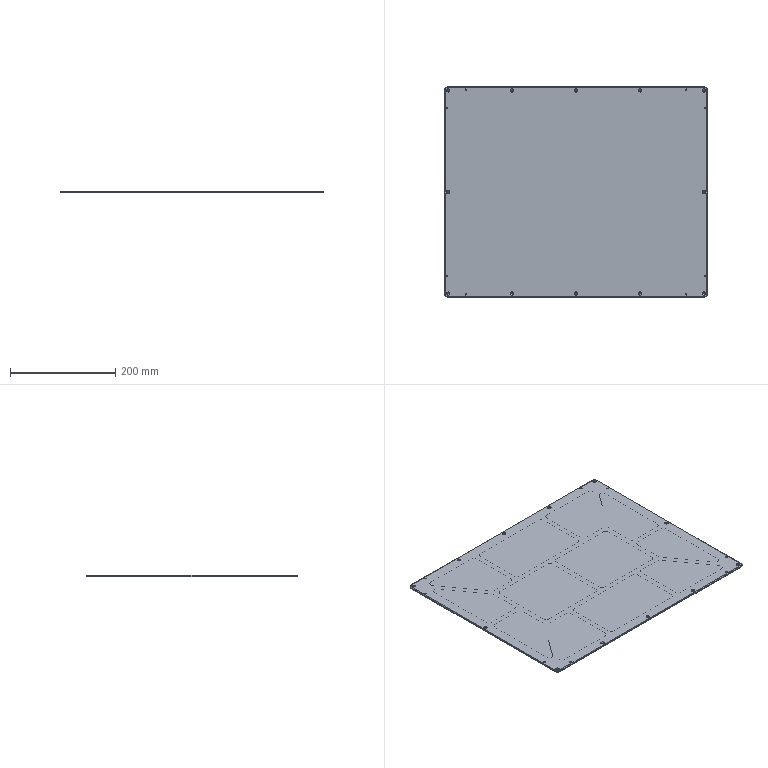NC program | Mastercam | posted with a generic post | part box 500 x 400 x 3 mm
Lines 2042 to 3034 of 11256:
(8 FEM |TOOL - 8|DIA. OFF. - 8|LEN. - 8|TOOL DIA. - 8.)
N4158 T8 M6
N4160 G0 G54 G90 X-136.27 Y140.355 C0. B0. S7000 M3
N4162 G43 H8 Z50.
N4164 Z1.
N4166 G1 Z.333 F600.
N4168 X-138.465 Z.314 F3500.
N4170 X-140.67 Z.295
N4172 X-145.964 Z.257
N4174 X-143.536 Y137.017
N4176 X-140.948 Y133.459 Z.219
N4178 X-138.36 Y129.9 Z.181
N4180 X-134.645 Y124.791 Z.144
N4182 Y127.543
N4184 Y131.943 Z.106
N4186 Y136.343 Z.068
N4188 Y140.355 Z.033
N4190 X-136.452 Z.03
N4192 X-138.465 Z.012
N4194 X-140.852 Z-.008
N4196 X-145.964 Z-.046
N4198 X-145.081 Y139.141
N4200 X-142.493 Y135.583 Z-.084
N4202 X-139.906 Y132.025 Z-.122
N4204 X-137.318 Y128.466 Z-.16
N4206 X-134.645 Y124.791 Z-.198
N4208 Y124.971
N4210 Y129.371 Z-.236
N4212 Y133.771 Z-.274
N4214 Y138.171 Z-.312
N4216 Y140.355 Z-.331
N4218 X-138.465 Z-.35
N4220 G3 X-139.29 Y139.53 J-.825
N4222 X-139.262 Y139.318 I.825
N4224 G1 X-138.595 Y136.809
N4226 G3 X-138.465 Y136.536 I.798 J.212
N4228 G2 X-139.246 Y137.097 J.825
N4230 G1 X-140.158 Y139.794
N4232 G3 X-140.94 Y140.355 I-.782 J-.264
N4234 G1 X-145.964
N4236 X-134.645 Y124.791
N4238 Y140.355
N4240 X-140.94
N4242 G2 X-141.729 Y140.941 J.825
N4244 G1 X-142.625 Y143.904
N4246 G3 X-143.415 Y144.49 I-.79 J-.239
N4248 G1 X-154.084
N4250 X-130.51 Y112.075
N4252 Y144.49
N4254 X-143.415
N4256 G2 X-144.207 Y145.085 J.825
N4258 G1 X-145.097 Y148.154
N4260 G3 X-145.89 Y148.749 I-.793 J-.23
N4262 G1 X-162.447
N4264 X-131.54 Y106.251
N4266 X-126.251
N4268 Y148.749
N4270 X-145.89
N4272 G2 X-146.687 Y149.361 J.825
N4274 G1 X-147.567 Y152.662
N4276 G3 X-148.365 Y153.274 I-.798 J-.213
N4278 G1 X-171.334
N4280 X-133.844 Y101.726
N4282 X-121.726
N4284 Y153.274
N4286 X-148.365
N4288 G2 X-149.162 Y153.886 J.825
N4290 G1 X-150.042 Y157.187
N4292 G3 X-150.84 Y157.799 I-.798 J-.213
N4294 G1 X-180.22
N4296 X-136.149 Y97.201
N4298 X-117.201
N4300 Y157.799
N4302 X-150.84
N4304 G2 X-151.637 Y158.411 J.825
N4306 G1 X-152.517 Y161.712
N4308 G3 X-153.315 Y162.324 I-.798 J-.213
N4310 G1 X-189.106
N4312 X-138.453 Y92.676
N4314 X-112.676
N4316 Y162.324
N4318 X-153.315
N4320 G2 X-154.112 Y162.937 J.825
N4322 G1 X-154.992 Y166.237
N4324 G3 X-155.79 Y166.85 I-.798 J-.212
N4326 G1 X-197.993
N4328 X-140.757 Y88.15
N4330 X-108.15
N4332 Y166.85
N4334 X-155.79
N4336 G2 X-156.587 Y167.462 J.825
N4338 G1 X-157.467 Y170.762
N4340 G3 X-158.265 Y171.375 I-.798 J-.212
N4342 G1 X-206.88
N4344 X-143.062 Y83.625
N4346 X-103.625
N4348 Y171.375
N4350 X-158.265
N4352 G2 X-159.062 Y171.987 J.825
N4354 G1 X-159.942 Y175.288
N4356 G3 X-160.74 Y175.9 I-.798 J-.213
N4358 G1 X-210.496
N4360 X-211.127 Y175.879
N4362 X-211.757 Y175.773
N4364 G3 X-212.449 Y175.426 I1.634 J-4.119
N4366 X-213.433 Y173.534 I1.398 J-1.929
N4368 G1 X-213.357 Y172.903
N4370 X-213.245 Y172.579
N4372 G3 X-212.669 Y171.642 I9.36 J5.107
N4374 G1 X-146.185 Y80.226
N4376 X-145.554 Y79.574
N4378 G3 X-144.613 Y79.165 I1.565 J2.311
N4380 G1 X-143.663 Y79.1
N4382 X-102.05
N4384 X-101.419 Y79.122
N4386 X-100.789 Y79.231
N4388 G3 X-100.108 Y79.574 I-1.685 J4.186
N4390 X-99.34 Y80.51 I-1.549 J2.054
N4392 G1 X-99.219 Y80.835
N4394 X-99.118 Y81.466
N4396 X-99.1 Y172.903
N4398 X-99.118 Y173.534
N4400 X-99.219 Y174.165
N4402 G3 X-99.791 Y175.151 I-2.451 J-.764
N4404 X-100.789 Y175.769 I-1.843 J-1.86
N4406 G1 X-101.419 Y175.878
N4408 X-102.05 Y175.9
N4410 X-160.74
N4412 G0 Z50.
N4414 X-136.27 Y140.355
N4416 Z.65
N4418 G1 Z-.017 F600.
N4420 X-138.465 Z-.036 F3500.
N4422 X-140.67 Z-.055
N4424 X-145.964 Z-.093
N4426 X-143.536 Y137.017
N4428 X-140.948 Y133.459 Z-.131
N4430 X-138.36 Y129.9 Z-.169
N4432 X-134.645 Y124.791 Z-.206
N4434 Y127.543
N4436 Y131.943 Z-.244
N4438 Y136.343 Z-.282
N4440 Y140.355 Z-.317
N4442 X-136.452 Z-.32
N4444 X-138.465 Z-.338
N4446 X-140.852 Z-.358
N4448 X-145.964 Z-.396
N4450 X-145.081 Y139.141
N4452 X-142.493 Y135.583 Z-.434
N4454 X-139.906 Y132.025 Z-.472
N4456 X-137.318 Y128.466 Z-.51
N4458 X-134.645 Y124.791 Z-.548
N4460 Y124.971
N4462 Y129.371 Z-.586
N4464 Y133.771 Z-.624
N4466 Y138.171 Z-.662
N4468 Y140.355 Z-.681
N4470 X-138.465 Z-.7
N4472 G3 X-139.29 Y139.53 J-.825
N4474 X-139.262 Y139.318 I.825
N4476 G1 X-138.595 Y136.809
N4478 G3 X-138.465 Y136.536 I.798 J.212
N4480 G2 X-139.246 Y137.097 J.825
N4482 G1 X-140.158 Y139.794
N4484 G3 X-140.94 Y140.355 I-.782 J-.264
N4486 G1 X-145.964
N4488 X-134.645 Y124.791
N4490 Y140.355
N4492 X-140.94
N4494 G2 X-141.729 Y140.941 J.825
N4496 G1 X-142.625 Y143.904
N4498 G3 X-143.415 Y144.49 I-.79 J-.239
N4500 G1 X-154.084
N4502 X-130.51 Y112.075
N4504 Y144.49
N4506 X-143.415
N4508 G2 X-144.207 Y145.085 J.825
N4510 G1 X-145.097 Y148.154
N4512 G3 X-145.89 Y148.749 I-.793 J-.23
N4514 G1 X-162.447
N4516 X-131.54 Y106.251
N4518 X-126.251
N4520 Y148.749
N4522 X-145.89
N4524 G2 X-146.687 Y149.361 J.825
N4526 G1 X-147.567 Y152.662
N4528 G3 X-148.365 Y153.274 I-.798 J-.213
N4530 G1 X-171.334
N4532 X-133.844 Y101.726
N4534 X-121.726
N4536 Y153.274
N4538 X-148.365
N4540 G2 X-149.162 Y153.886 J.825
N4542 G1 X-150.042 Y157.187
N4544 G3 X-150.84 Y157.799 I-.798 J-.213
N4546 G1 X-180.22
N4548 X-136.149 Y97.201
N4550 X-117.201
N4552 Y157.799
N4554 X-150.84
N4556 G2 X-151.637 Y158.411 J.825
N4558 G1 X-152.517 Y161.712
N4560 G3 X-153.315 Y162.324 I-.798 J-.213
N4562 G1 X-189.106
N4564 X-138.453 Y92.676
N4566 X-112.676
N4568 Y162.324
N4570 X-153.315
N4572 G2 X-154.112 Y162.937 J.825
N4574 G1 X-154.992 Y166.237
N4576 G3 X-155.79 Y166.85 I-.798 J-.212
N4578 G1 X-197.993
N4580 X-140.757 Y88.15
N4582 X-108.15
N4584 Y166.85
N4586 X-155.79
N4588 G2 X-156.587 Y167.462 J.825
N4590 G1 X-157.467 Y170.762
N4592 G3 X-158.265 Y171.375 I-.798 J-.212
N4594 G1 X-206.88
N4596 X-143.062 Y83.625
N4598 X-103.625
N4600 Y171.375
N4602 X-158.265
N4604 G2 X-159.062 Y171.987 J.825
N4606 G1 X-159.942 Y175.288
N4608 G3 X-160.74 Y175.9 I-.798 J-.213
N4610 G1 X-210.496
N4612 X-211.127 Y175.879
N4614 X-211.757 Y175.773
N4616 G3 X-212.449 Y175.426 I1.634 J-4.119
N4618 X-213.433 Y173.534 I1.398 J-1.929
N4620 G1 X-213.357 Y172.903
N4622 X-213.245 Y172.579
N4624 G3 X-212.669 Y171.642 I9.36 J5.107
N4626 G1 X-146.185 Y80.226
N4628 X-145.554 Y79.574
N4630 G3 X-144.613 Y79.165 I1.565 J2.311
N4632 G1 X-143.663 Y79.1
N4634 X-102.05
N4636 X-101.419 Y79.122
N4638 X-100.789 Y79.231
N4640 G3 X-100.108 Y79.574 I-1.685 J4.186
N4642 X-99.34 Y80.51 I-1.549 J2.054
N4644 G1 X-99.219 Y80.835
N4646 X-99.118 Y81.466
N4648 X-99.1 Y172.903
N4650 X-99.118 Y173.534
N4652 X-99.219 Y174.165
N4654 G3 X-99.791 Y175.151 I-2.451 J-.764
N4656 X-100.789 Y175.769 I-1.843 J-1.86
N4658 G1 X-101.419 Y175.878
N4660 X-102.05 Y175.9
N4662 X-160.74
N4664 G0 Z50.
N4666 X-136.27 Y140.355
N4668 Z.3
N4670 G1 Z-.367 F600.
N4672 X-138.465 Z-.386 F3500.
N4674 X-140.67 Z-.405
N4676 X-145.964 Z-.443
N4678 X-143.536 Y137.017
N4680 X-140.948 Y133.459 Z-.481
N4682 X-138.36 Y129.9 Z-.519
N4684 X-134.645 Y124.791 Z-.556
N4686 Y127.543
N4688 Y131.943 Z-.594
N4690 Y136.343 Z-.632
N4692 Y140.355 Z-.667
N4694 X-136.452 Z-.67
N4696 X-138.465 Z-.688
N4698 X-140.852 Z-.708
N4700 X-145.964 Z-.746
N4702 X-145.081 Y139.141
N4704 X-142.493 Y135.583 Z-.784
N4706 X-139.906 Y132.025 Z-.822
N4708 X-137.318 Y128.466 Z-.86
N4710 X-134.645 Y124.791 Z-.898
N4712 Y124.971
N4714 Y129.371 Z-.936
N4716 Y133.771 Z-.974
N4718 Y138.171 Z-1.012
N4720 Y140.355 Z-1.031
N4722 X-138.465 Z-1.05
N4724 G3 X-139.29 Y139.53 J-.825
N4726 X-139.262 Y139.318 I.825
N4728 G1 X-138.595 Y136.809
N4730 G3 X-138.465 Y136.536 I.798 J.212
N4732 G2 X-139.246 Y137.097 J.825
N4734 G1 X-140.158 Y139.794
N4736 G3 X-140.94 Y140.355 I-.782 J-.264
N4738 G1 X-145.964
N4740 X-134.645 Y124.791
N4742 Y140.355
N4744 X-140.94
N4746 G2 X-141.729 Y140.941 J.825
N4748 G1 X-142.625 Y143.904
N4750 G3 X-143.415 Y144.49 I-.79 J-.239
N4752 G1 X-154.084
N4754 X-130.51 Y112.075
N4756 Y144.49
N4758 X-143.415
N4760 G2 X-144.207 Y145.085 J.825
N4762 G1 X-145.097 Y148.154
N4764 G3 X-145.89 Y148.749 I-.793 J-.23
N4766 G1 X-162.447
N4768 X-131.54 Y106.251
N4770 X-126.251
N4772 Y148.749
N4774 X-145.89
N4776 G2 X-146.687 Y149.361 J.825
N4778 G1 X-147.567 Y152.662
N4780 G3 X-148.365 Y153.274 I-.798 J-.213
N4782 G1 X-171.334
N4784 X-133.844 Y101.726
N4786 X-121.726
N4788 Y153.274
N4790 X-148.365
N4792 G2 X-149.162 Y153.886 J.825
N4794 G1 X-150.042 Y157.187
N4796 G3 X-150.84 Y157.799 I-.798 J-.213
N4798 G1 X-180.22
N4800 X-136.149 Y97.201
N4802 X-117.201
N4804 Y157.799
N4806 X-150.84
N4808 G2 X-151.637 Y158.411 J.825
N4810 G1 X-152.517 Y161.712
N4812 G3 X-153.315 Y162.324 I-.798 J-.213
N4814 G1 X-189.106
N4816 X-138.453 Y92.676
N4818 X-112.676
N4820 Y162.324
N4822 X-153.315
N4824 G2 X-154.112 Y162.937 J.825
N4826 G1 X-154.992 Y166.237
N4828 G3 X-155.79 Y166.85 I-.798 J-.212
N4830 G1 X-197.993
N4832 X-140.757 Y88.15
N4834 X-108.15
N4836 Y166.85
N4838 X-155.79
N4840 G2 X-156.587 Y167.462 J.825
N4842 G1 X-157.467 Y170.762
N4844 G3 X-158.265 Y171.375 I-.798 J-.212
N4846 G1 X-206.88
N4848 X-143.062 Y83.625
N4850 X-103.625
N4852 Y171.375
N4854 X-158.265
N4856 G2 X-159.062 Y171.987 J.825
N4858 G1 X-159.942 Y175.288
N4860 G3 X-160.74 Y175.9 I-.798 J-.213
N4862 G1 X-210.496
N4864 X-211.127 Y175.879
N4866 X-211.757 Y175.773
N4868 G3 X-212.449 Y175.426 I1.634 J-4.119
N4870 X-213.433 Y173.534 I1.398 J-1.929
N4872 G1 X-213.357 Y172.903
N4874 X-213.245 Y172.579
N4876 G3 X-212.669 Y171.642 I9.36 J5.107
N4878 G1 X-146.185 Y80.226
N4880 X-145.554 Y79.574
N4882 G3 X-144.613 Y79.165 I1.565 J2.311
N4884 G1 X-143.663 Y79.1
N4886 X-102.05
N4888 X-101.419 Y79.122
N4890 X-100.789 Y79.231
N4892 G3 X-100.108 Y79.574 I-1.685 J4.186
N4894 X-99.34 Y80.51 I-1.549 J2.054
N4896 G1 X-99.219 Y80.835
N4898 X-99.118 Y81.466
N4900 X-99.1 Y172.903
N4902 X-99.118 Y173.534
N4904 X-99.219 Y174.165
N4906 G3 X-99.791 Y175.151 I-2.451 J-.764
N4908 X-100.789 Y175.769 I-1.843 J-1.86
N4910 G1 X-101.419 Y175.878
N4912 X-102.05 Y175.9
N4914 X-160.74
N4916 G0 Z50.
N4918 X-136.27 Y140.355
N4920 Z-.05
N4922 G1 Z-.717 F600.
N4924 X-138.465 Z-.736 F3500.
N4926 X-140.67 Z-.755
N4928 X-145.964 Z-.793
N4930 X-143.536 Y137.017
N4932 X-140.948 Y133.459 Z-.831
N4934 X-138.36 Y129.9 Z-.869
N4936 X-134.645 Y124.791 Z-.906
N4938 Y127.543
N4940 Y131.943 Z-.944
N4942 Y136.343 Z-.982
N4944 Y140.355 Z-1.017
N4946 X-136.452 Z-1.02
N4948 X-138.465 Z-1.038
N4950 X-140.852 Z-1.058
N4952 X-145.964 Z-1.096
N4954 X-145.081 Y139.141
N4956 X-142.493 Y135.583 Z-1.134
N4958 X-139.906 Y132.025 Z-1.172
N4960 X-137.318 Y128.466 Z-1.21
N4962 X-134.645 Y124.791 Z-1.248
N4964 Y124.971
N4966 Y129.371 Z-1.286
N4968 Y133.771 Z-1.324
N4970 Y138.171 Z-1.362
N4972 Y140.355 Z-1.381
N4974 X-138.465 Z-1.4
N4976 G3 X-139.29 Y139.53 J-.825
N4978 X-139.262 Y139.318 I.825
N4980 G1 X-138.595 Y136.809
N4982 G3 X-138.465 Y136.536 I.798 J.212
N4984 G2 X-139.246 Y137.097 J.825
N4986 G1 X-140.158 Y139.794
N4988 G3 X-140.94 Y140.355 I-.782 J-.264
N4990 G1 X-145.964
N4992 X-134.645 Y124.791
N4994 Y140.355
N4996 X-140.94
N4998 G2 X-141.729 Y140.941 J.825
N5000 G1 X-142.625 Y143.904
N5002 G3 X-143.415 Y144.49 I-.79 J-.239
N5004 G1 X-154.084
N5006 X-130.51 Y112.075
N5008 Y144.49
N5010 X-143.415
N5012 G2 X-144.207 Y145.085 J.825
N5014 G1 X-145.097 Y148.154
N5016 G3 X-145.89 Y148.749 I-.793 J-.23
N5018 G1 X-162.447
N5020 X-131.54 Y106.251
N5022 X-126.251
N5024 Y148.749
N5026 X-145.89
N5028 G2 X-146.687 Y149.361 J.825
N5030 G1 X-147.567 Y152.662
N5032 G3 X-148.365 Y153.274 I-.798 J-.213
N5034 G1 X-171.334
N5036 X-133.844 Y101.726
N5038 X-121.726
N5040 Y153.274
N5042 X-148.365
N5044 G2 X-149.162 Y153.886 J.825
N5046 G1 X-150.042 Y157.187
N5048 G3 X-150.84 Y157.799 I-.798 J-.213
N5050 G1 X-180.22
N5052 X-136.149 Y97.201
N5054 X-117.201
N5056 Y157.799
N5058 X-150.84
N5060 G2 X-151.637 Y158.411 J.825
N5062 G1 X-152.517 Y161.712
N5064 G3 X-153.315 Y162.324 I-.798 J-.213
N5066 G1 X-189.106
N5068 X-138.453 Y92.676
N5070 X-112.676
N5072 Y162.324
N5074 X-153.315
N5076 G2 X-154.112 Y162.937 J.825
N5078 G1 X-154.992 Y166.237
N5080 G3 X-155.79 Y166.85 I-.798 J-.212
N5082 G1 X-197.993
N5084 X-140.757 Y88.15
N5086 X-108.15
N5088 Y166.85
N5090 X-155.79
N5092 G2 X-156.587 Y167.462 J.825
N5094 G1 X-157.467 Y170.762
N5096 G3 X-158.265 Y171.375 I-.798 J-.212
N5098 G1 X-206.88
N5100 X-143.062 Y83.625
N5102 X-103.625
N5104 Y171.375
N5106 X-158.265
N5108 G2 X-159.062 Y171.987 J.825
N5110 G1 X-159.942 Y175.288
N5112 G3 X-160.74 Y175.9 I-.798 J-.213
N5114 G1 X-210.496
N5116 X-211.127 Y175.879
N5118 X-211.757 Y175.773
N5120 G3 X-212.449 Y175.426 I1.634 J-4.119
N5122 X-213.433 Y173.534 I1.398 J-1.929
N5124 G1 X-213.357 Y172.903
N5126 X-213.245 Y172.579
N5128 G3 X-212.669 Y171.642 I9.36 J5.107
N5130 G1 X-146.185 Y80.226
N5132 X-145.554 Y79.574
N5134 G3 X-144.613 Y79.165 I1.565 J2.311
N5136 G1 X-143.663 Y79.1
N5138 X-102.05
N5140 X-101.419 Y79.122
N5142 X-100.789 Y79.231
N5144 G3 X-100.108 Y79.574 I-1.685 J4.186
N5146 X-99.34 Y80.51 I-1.549 J2.054
N5148 G1 X-99.219 Y80.835
N5150 X-99.118 Y81.466
N5152 X-99.1 Y172.903
N5154 X-99.118 Y173.534
N5156 X-99.219 Y174.165
N5158 G3 X-99.791 Y175.151 I-2.451 J-.764
N5160 X-100.789 Y175.769 I-1.843 J-1.86
N5162 G1 X-101.419 Y175.878
N5164 X-102.05 Y175.9
N5166 X-160.74
N5168 G0 Z50.
N5170 X-136.27 Y140.355
N5172 Z-.4
N5174 G1 Z-.817 F600.
N5176 X-138.465 Z-.836 F1000.
N5178 X-140.67 Z-.855
N5180 X-145.964 Z-.893
N5182 X-143.536 Y137.017
N5184 X-140.948 Y133.459 Z-.931
N5186 X-138.36 Y129.9 Z-.969
N5188 X-134.645 Y124.791 Z-1.006
N5190 Y127.543
N5192 Y131.943 Z-1.044
N5194 Y136.343 Z-1.082
N5196 Y140.355 Z-1.117
N5198 X-136.452 Z-1.12
N5200 X-138.465 Z-1.138
N5202 X-140.852 Z-1.158
N5204 X-145.964 Z-1.196
N5206 X-145.081 Y139.141
N5208 X-142.493 Y135.583 Z-1.234
N5210 X-139.906 Y132.025 Z-1.272
N5212 X-137.318 Y128.466 Z-1.31
N5214 X-134.645 Y124.791 Z-1.348
N5216 Y124.971
N5218 Y129.371 Z-1.386
N5220 Y133.771 Z-1.424
N5222 Y138.171 Z-1.462
N5224 Y140.355 Z-1.481
N5226 X-138.465 Z-1.5
N5228 G3 X-139.29 Y139.53 J-.825 F3500.
N5230 X-139.262 Y139.318 I.825
N5232 G1 X-138.595 Y136.809
N5234 G3 X-138.465 Y136.536 I.798 J.212
N5236 G2 X-139.246 Y137.097 J.825
N5238 G1 X-140.158 Y139.794
N5240 G3 X-140.94 Y140.355 I-.782 J-.264
N5242 G1 X-145.964 F1000.
N5244 X-134.645 Y124.791
N5246 Y140.355
N5248 X-140.94
N5250 G2 X-141.729 Y140.941 J.825 F3500.
N5252 G1 X-142.625 Y143.904
N5254 G3 X-143.415 Y144.49 I-.79 J-.239
N5256 G1 X-154.084 F1000.
N5258 X-130.51 Y112.075
N5260 Y144.49
N5262 X-143.415
N5264 G2 X-144.207 Y145.085 J.825 F3500.
N5266 G1 X-145.097 Y148.154
N5268 G3 X-145.89 Y148.749 I-.793 J-.23
N5270 G1 X-162.447 F1000.
N5272 X-131.54 Y106.251
N5274 X-126.251
N5276 Y148.749
N5278 X-145.89
N5280 G2 X-146.687 Y149.361 J.825 F3500.
N5282 G1 X-147.567 Y152.662
N5284 G3 X-148.365 Y153.274 I-.798 J-.213
N5286 G1 X-171.334 F1000.
N5288 X-133.844 Y101.726
N5290 X-121.726
N5292 Y153.274
N5294 X-148.365
N5296 G2 X-149.162 Y153.886 J.825 F3500.
N5298 G1 X-150.042 Y157.187
N5300 G3 X-150.84 Y157.799 I-.798 J-.213
N5302 G1 X-180.22 F1000.
N5304 X-136.149 Y97.201
N5306 X-117.201
N5308 Y157.799
N5310 X-150.84
N5312 G2 X-151.637 Y158.411 J.825 F3500.
N5314 G1 X-152.517 Y161.712
N5316 G3 X-153.315 Y162.324 I-.798 J-.213
N5318 G1 X-189.106 F1000.
N5320 X-138.453 Y92.676
N5322 X-112.676
N5324 Y162.324
N5326 X-153.315
N5328 G2 X-154.112 Y162.937 J.825 F3500.
N5330 G1 X-154.992 Y166.237
N5332 G3 X-155.79 Y166.85 I-.798 J-.212
N5334 G1 X-197.993 F1000.
N5336 X-140.757 Y88.15
N5338 X-108.15
N5340 Y166.85
N5342 X-155.79
N5344 G2 X-156.587 Y167.462 J.825 F3500.
N5346 G1 X-157.467 Y170.762
N5348 G3 X-158.265 Y171.375 I-.798 J-.212
N5350 G1 X-206.88 F1000.
N5352 X-143.062 Y83.625
N5354 X-103.625
N5356 Y171.375
N5358 X-158.265
N5360 G2 X-159.062 Y171.987 J.825 F3500.
N5362 G1 X-159.942 Y175.288
N5364 G3 X-160.74 Y175.9 I-.798 J-.213
N5366 G1 X-210.496 F1000.
N5368 X-211.127 Y175.879
N5370 X-211.757 Y175.773
N5372 G3 X-212.449 Y175.426 I1.634 J-4.119
N5374 X-213.433 Y173.534 I1.398 J-1.929
N5376 G1 X-213.357 Y172.903
N5378 X-213.245 Y172.579
N5380 G3 X-212.669 Y171.642 I9.36 J5.107
N5382 G1 X-146.185 Y80.226
N5384 X-145.554 Y79.574
N5386 G3 X-144.613 Y79.165 I1.565 J2.311
N5388 G1 X-143.663 Y79.1
N5390 X-102.05
N5392 X-101.419 Y79.122
N5394 X-100.789 Y79.231
N5396 G3 X-100.108 Y79.574 I-1.685 J4.186
N5398 X-99.34 Y80.51 I-1.549 J2.054
N5400 G1 X-99.219 Y80.835
N5402 X-99.118 Y81.466
N5404 X-99.1 Y172.903
N5406 X-99.118 Y173.534
N5408 X-99.219 Y174.165
N5410 G3 X-99.791 Y175.151 I-2.451 J-.764
N5412 X-100.789 Y175.769 I-1.843 J-1.86
N5414 G1 X-101.419 Y175.878
N5416 X-102.05 Y175.9
N5418 X-160.74
N5420 G0 Z50.
N5422 X-10.062 Y125.983
N5424 Z1.
N5426 G1 Z.333 F600.
N5428 X-5.662 Z.295 F3500.
N5430 X-1.262 Z.257
N5432 X3.138 Z.219
N5434 X7.538 Z.181
N5436 X11.938 Z.144
N5438 X16.338 Z.106
N5440 X20.738 Z.068
N5442 X25.138 Z.03
N5444 X29.538 Z-.008
N5446 X34.017 Z-.046
N5448 Y129.017
N5450 X32.725
N5452 X28.325 Z-.084
N5454 X23.925 Z-.122
N5456 X19.525 Z-.16
N5458 X15.125 Z-.198
N5460 X10.725 Z-.236
N5462 X6.325 Z-.274
N5464 X1.925 Z-.312
N5466 X0. Z-.329
N5468 X-2.475 Z-.35
N5470 X-34.017
N5472 Y125.983
N5474 X34.017
N5476 Y129.017
N5478 X0.
N5480 X-2.475
N5482 G2 X-3.281 Y129.664 J.825
N5484 G1 X-4.144 Y133.579
N5486 G3 X-4.95 Y134.226 I-.806 J-.178
N5488 G1 X-39.226
N5490 Y120.774
N5492 X39.226
N5494 Y134.226
N5496 X0.
N5498 X-4.95
N5500 G2 X-5.756 Y134.873 J.825
N5502 G1 X-6.619 Y138.788
N5504 G3 X-7.425 Y139.435 I-.806 J-.178
N5506 G1 X-44.435
N5508 Y115.565
N5510 X44.435
N5512 Y139.435
N5514 X0.
N5516 X-7.425
N5518 G2 X-8.231 Y140.083 J.825
N5520 G1 X-9.094 Y143.998
N5522 G3 X-9.9 Y144.645 I-.806 J-.178
N5524 G1 X-49.645
N5526 Y110.355
N5528 X49.645
N5530 Y144.645
N5532 X0.
N5534 X-9.9
N5536 G2 X-10.706 Y145.292 J.825
N5538 G1 X-11.569 Y149.207
N5540 G3 X-12.375 Y149.854 I-.806 J-.178
N5542 G1 X-54.854
N5544 Y105.146
N5546 X54.854
N5548 Y149.854
N5550 X0.
N5552 X-12.375
N5554 G2 X-13.181 Y150.501 J.825
N5556 G1 X-14.044 Y154.416
N5558 G3 X-14.85 Y155.063 I-.806 J-.178
N5560 G1 X-60.063
N5562 Y99.937
N5564 X60.063
N5566 Y155.063
N5568 X0.
N5570 X-14.85
N5572 G2 X-15.656 Y155.711 J.825
N5574 G1 X-16.519 Y159.625
N5576 G3 X-17.325 Y160.273 I-.806 J-.177
N5578 G1 X-65.273
N5580 Y94.727
N5582 X65.273
N5584 Y160.273
N5586 X0.
N5588 X-17.325
N5590 G2 X-18.131 Y160.92 J.825
N5592 G1 X-18.994 Y164.834
N5594 G3 X-19.8 Y165.482 I-.806 J-.177
N5596 G1 X-70.482
N5598 Y89.518
N5600 X70.482
N5602 Y165.482
N5604 X0.
N5606 X-19.8
N5608 G2 X-20.606 Y166.129 J.825
N5610 G1 X-21.469 Y170.044
N5612 G3 X-22.275 Y170.691 I-.806 J-.178
N5614 G1 X-75.691
N5616 Y84.309
N5618 X75.691
N5620 Y170.691
N5622 X0.
N5624 X-22.275
N5626 G2 X-23.081 Y171.338 J.825
N5628 G1 X-23.944 Y175.253
N5630 G3 X-24.75 Y175.9 I-.806 J-.178
N5632 G1 X-78.199
N5634 X-78.83 Y175.856
N5636 X-79.314 Y175.741
N5638 G3 X-80.091 Y175.269 I1.466 J-3.285
N5640 X-80.722 Y174.357 I1.955 J-2.027
N5642 X-80.9 Y173.221 I3.526 J-1.136
N5644 G1 Y173.219
N5646 Y81.781
N5648 Y81.779
N5650 G3 X-80.722 Y80.643 I3.704
N5652 X-80.091 Y79.731 I2.586 J1.115
N5654 X-79.314 Y79.259 I2.243 J2.813
N5656 G1 X-78.83 Y79.144
N5658 X-78.199 Y79.1
N5660 X78.199
N5662 X78.83 Y79.144
N5664 X79.314 Y79.259
N5666 G3 X80.091 Y79.731 I-1.466 J3.285
N5668 X80.722 Y80.643 I-1.955 J2.027
N5670 X80.9 Y81.779 I-3.526 J1.136
N5672 G1 Y81.781
N5674 Y173.219
N5676 Y173.221
N5678 G3 X80.722 Y174.357 I-3.704
N5680 X80.091 Y175.269 I-2.586 J-1.115
N5682 X79.314 Y175.741 I-2.243 J-2.813
N5684 G1 X78.83 Y175.856
N5686 X78.199 Y175.9
N5688 X0.
N5690 X-24.75
N5692 G0 Z50.
N5694 X-10.062 Y125.983
N5696 Z.65
N5698 G1 Z-.017 F600.
N5700 X-5.662 Z-.055 F3500.
N5702 X-1.262 Z-.093
N5704 X3.138 Z-.131
N5706 X7.538 Z-.169
N5708 X11.938 Z-.206
N5710 X16.338 Z-.244
N5712 X20.738 Z-.282
N5714 X25.138 Z-.32
N5716 X29.538 Z-.358
N5718 X34.017 Z-.396
N5720 Y129.017
N5722 X32.725
N5724 X28.325 Z-.434
N5726 X23.925 Z-.472
N5728 X19.525 Z-.51
N5730 X15.125 Z-.548
N5732 X10.725 Z-.586
N5734 X6.325 Z-.624
N5736 X1.925 Z-.662
N5738 X0. Z-.679
N5740 X-2.475 Z-.7
N5742 X-34.017
N5744 Y125.983
N5746 X34.017
N5748 Y129.017
N5750 X0.
N5752 X-2.475
N5754 G2 X-3.281 Y129.664 J.825
N5756 G1 X-4.144 Y133.579
N5758 G3 X-4.95 Y134.226 I-.806 J-.178
N5760 G1 X-39.226
N5762 Y120.774
N5764 X39.226
N5766 Y134.226
N5768 X0.
N5770 X-4.95
N5772 G2 X-5.756 Y134.873 J.825
N5774 G1 X-6.619 Y138.788
N5776 G3 X-7.425 Y139.435 I-.806 J-.178
N5778 G1 X-44.435
N5780 Y115.565
N5782 X44.435
N5784 Y139.435
N5786 X0.
N5788 X-7.425
N5790 G2 X-8.231 Y140.083 J.825
N5792 G1 X-9.094 Y143.998
N5794 G3 X-9.9 Y144.645 I-.806 J-.178
N5796 G1 X-49.645
N5798 Y110.355
N5800 X49.645
N5802 Y144.645
N5804 X0.
N5806 X-9.9
N5808 G2 X-10.706 Y145.292 J.825
N5810 G1 X-11.569 Y149.207
N5812 G3 X-12.375 Y149.854 I-.806 J-.178
N5814 G1 X-54.854
N5816 Y105.146
N5818 X54.854
N5820 Y149.854
N5822 X0.
N5824 X-12.375
N5826 G2 X-13.181 Y150.501 J.825
N5828 G1 X-14.044 Y154.416
N5830 G3 X-14.85 Y155.063 I-.806 J-.178
N5832 G1 X-60.063
N5834 Y99.937
N5836 X60.063
N5838 Y155.063
N5840 X0.
N5842 X-14.85
N5844 G2 X-15.656 Y155.711 J.825
N5846 G1 X-16.519 Y159.625
N5848 G3 X-17.325 Y160.273 I-.806 J-.177
N5850 G1 X-65.273
N5852 Y94.727
N5854 X65.273
N5856 Y160.273
N5858 X0.
N5860 X-17.325
N5862 G2 X-18.131 Y160.92 J.825
N5864 G1 X-18.994 Y164.834
N5866 G3 X-19.8 Y165.482 I-.806 J-.177
N5868 G1 X-70.482
N5870 Y89.518
N5872 X70.482
N5874 Y165.482
N5876 X0.
N5878 X-19.8
N5880 G2 X-20.606 Y166.129 J.825
N5882 G1 X-21.469 Y170.044
N5884 G3 X-22.275 Y170.691 I-.806 J-.178
N5886 G1 X-75.691
N5888 Y84.309
N5890 X75.691
N5892 Y170.691
N5894 X0.
N5896 X-22.275
N5898 G2 X-23.081 Y171.338 J.825
N5900 G1 X-23.944 Y175.253
N5902 G3 X-24.75 Y175.9 I-.806 J-.178
N5904 G1 X-78.199
N5906 X-78.83 Y175.856
N5908 X-79.314 Y175.741
N5910 G3 X-80.091 Y175.269 I1.466 J-3.285
N5912 X-80.722 Y174.357 I1.955 J-2.027
N5914 X-80.9 Y173.221 I3.526 J-1.136
N5916 G1 Y173.219
N5918 Y81.781
N5920 Y81.779
N5922 G3 X-80.722 Y80.643 I3.704
N5924 X-80.091 Y79.731 I2.586 J1.115
N5926 X-79.314 Y79.259 I2.243 J2.813
N5928 G1 X-78.83 Y79.144
N5930 X-78.199 Y79.1
N5932 X78.199
N5934 X78.83 Y79.144
N5936 X79.314 Y79.259
N5938 G3 X80.091 Y79.731 I-1.466 J3.285
N5940 X80.722 Y80.643 I-1.955 J2.027
N5942 X80.9 Y81.779 I-3.526 J1.136
N5944 G1 Y81.781
N5946 Y173.219
N5948 Y173.221
N5950 G3 X80.722 Y174.357 I-3.704
N5952 X80.091 Y175.269 I-2.586 J-1.115
N5954 X79.314 Y175.741 I-2.243 J-2.813
N5956 G1 X78.83 Y175.856
N5958 X78.199 Y175.9
N5960 X0.
N5962 X-24.75
N5964 G0 Z50.
N5966 X-10.062 Y125.983
N5968 Z.3
N5970 G1 Z-.367 F600.
N5972 X-5.662 Z-.405 F3500.
N5974 X-1.262 Z-.443
N5976 X3.138 Z-.481
N5978 X7.538 Z-.519
N5980 X11.938 Z-.556
N5982 X16.338 Z-.594
N5984 X20.738 Z-.632
N5986 X25.138 Z-.67
N5988 X29.538 Z-.708
N5990 X34.017 Z-.746
N5992 Y129.017
N5994 X32.725
N5996 X28.325 Z-.784
N5998 X23.925 Z-.822
N6000 X19.525 Z-.86
N6002 X15.125 Z-.898
N6004 X10.725 Z-.936
N6006 X6.325 Z-.974
N6008 X1.925 Z-1.012
N6010 X0. Z-1.029
N6012 X-2.475 Z-1.05
N6014 X-34.017
N6016 Y125.983
N6018 X34.017
N6020 Y129.017
N6022 X0.
N6024 X-2.475
N6026 G2 X-3.281 Y129.664 J.825
N6028 G1 X-4.144 Y133.579
N6030 G3 X-4.95 Y134.226 I-.806 J-.178
N6032 G1 X-39.226
N6034 Y120.774
N6036 X39.226
N6038 Y134.226
N6040 X0.
N6042 X-4.95
N6044 G2 X-5.756 Y134.873 J.825
N6046 G1 X-6.619 Y138.788
N6048 G3 X-7.425 Y139.435 I-.806 J-.178
N6050 G1 X-44.435
N6052 Y115.565
N6054 X44.435
N6056 Y139.435
N6058 X0.
N6060 X-7.425
N6062 G2 X-8.231 Y140.083 J.825
N6064 G1 X-9.094 Y143.998
N6066 G3 X-9.9 Y144.645 I-.806 J-.178
N6068 G1 X-49.645
N6070 Y110.355
N6072 X49.645
N6074 Y144.645
N6076 X0.
N6078 X-9.9
N6080 G2 X-10.706 Y145.292 J.825
N6082 G1 X-11.569 Y149.207
N6084 G3 X-12.375 Y149.854 I-.806 J-.178
N6086 G1 X-54.854
N6088 Y105.146
N6090 X54.854
N6092 Y149.854
N6094 X0.
N6096 X-12.375
N6098 G2 X-13.181 Y150.501 J.825
N6100 G1 X-14.044 Y154.416
N6102 G3 X-14.85 Y155.063 I-.806 J-.178
N6104 G1 X-60.063
N6106 Y99.937
N6108 X60.063
N6110 Y155.063
N6112 X0.
N6114 X-14.85
N6116 G2 X-15.656 Y155.711 J.825
N6118 G1 X-16.519 Y159.625
N6120 G3 X-17.325 Y160.273 I-.806 J-.177
N6122 G1 X-65.273
N6124 Y94.727
N6126 X65.273
N6128 Y160.273
N6130 X0.
N6132 X-17.325
N6134 G2 X-18.131 Y160.92 J.825
N6136 G1 X-18.994 Y164.834
N6138 G3 X-19.8 Y165.482 I-.806 J-.177
N6140 G1 X-70.482